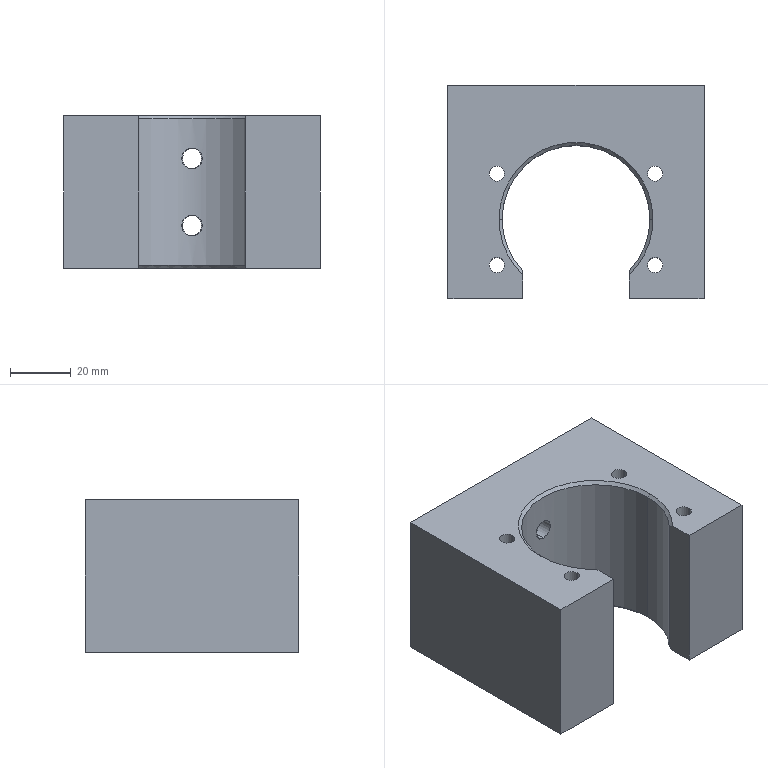Part | SolidWorks | features ICE 5, Chamfer 2, HoleWzd 2, Extrusion 1 | 1 solid | 50 faces | box 84 x 70 x 50 mm | volume 186072 mm3 | cylinder 23 | cone 18 | plane 9 | commonest cylinder face diameters 6.8 x12 5 x8 48.5 x3